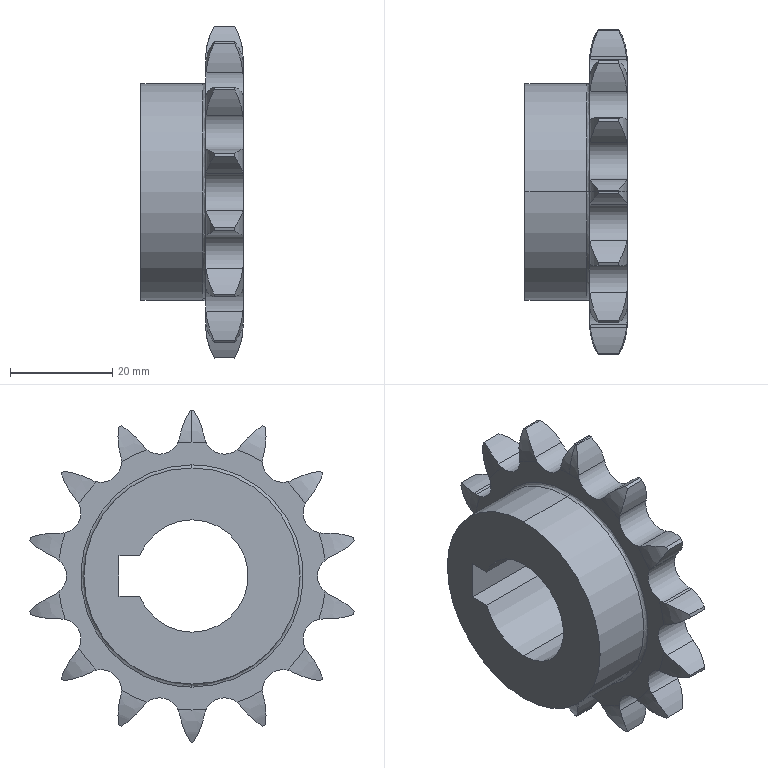Part | STEP file | short pitch roller chain wheel_s_iso_Chain wheel ISO - 14Z 08A-1 --14SB75H20L22.0R1 | 1 solid | 108 faces | box 20.001 x 63.542 x 65.028 mm | volume 26785 mm3 | cylinder 70 | spline 32 | plane 6 | commonest cylinder face diameters 30.413 x30 7.999 x20 65.028 x15 22 x3 42.33 x2